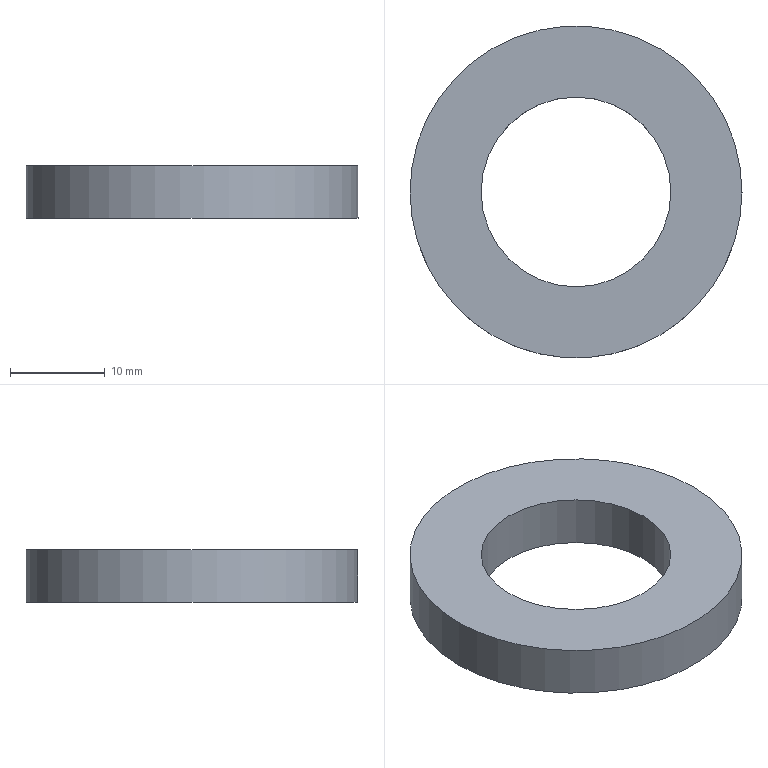Part | NX | 1 solid | 4 faces | box 35 x 35 x 5.5 mm | volume 3564 mm3 | plane 2 | cylinder 2 | commonest cylinder face diameters 20 x1 35 x1
STEP:
#1=CARTESIAN_POINT('',(17.5,0.,5.5));
#2=VERTEX_POINT('',#1);
#3=CARTESIAN_POINT('',(0.,0.,5.5));
#4=DIRECTION('',(0.,0.,1.));
#5=DIRECTION('',(1.,0.,0.));
#6=AXIS2_PLACEMENT_3D('',#3,#4,#5);
#7=CIRCLE('',#6,17.5);
#8=EDGE_CURVE('',#2,#2,#7,.T.);
#9=ORIENTED_EDGE('',*,*,#8,.T.);
#10=EDGE_LOOP('',(#9));
#11=FACE_BOUND('',#10,.T.);
#12=CARTESIAN_POINT('',(10.,0.,5.5));
#13=VERTEX_POINT('',#12);
#14=CARTESIAN_POINT('',(0.,0.,5.5));
#15=DIRECTION('',(0.,0.,1.));
#16=DIRECTION('',(1.,0.,0.));
#17=AXIS2_PLACEMENT_3D('',#14,#15,#16);
#18=CIRCLE('',#17,10.);
#19=EDGE_CURVE('',#13,#13,#18,.T.);
#20=ORIENTED_EDGE('',*,*,#19,.F.);
#21=EDGE_LOOP('',(#20));
#22=FACE_BOUND('',#21,.T.);
#23=CARTESIAN_POINT('',(0.,0.,5.5));
#24=DIRECTION('',(0.,0.,1.));
#25=DIRECTION('',(1.,0.,0.));
#26=AXIS2_PLACEMENT_3D('',#23,#24,#25);
#27=PLANE('',#26);
#28=ADVANCED_FACE('',(#11,#22),#27,.T.);
#29=CARTESIAN_POINT('',(17.5,0.,0.));
#30=VERTEX_POINT('',#29);
#31=CARTESIAN_POINT('',(0.,0.,0.));
#32=DIRECTION('',(0.,0.,1.));
#33=DIRECTION('',(1.,0.,0.));
#34=AXIS2_PLACEMENT_3D('',#31,#32,#33);
#35=CIRCLE('',#34,17.5);
#36=EDGE_CURVE('',#30,#30,#35,.T.);
#37=ORIENTED_EDGE('',*,*,#36,.F.);
#38=EDGE_LOOP('',(#37));
#39=FACE_BOUND('',#38,.T.);
#40=CARTESIAN_POINT('',(10.,0.,0.));
#41=VERTEX_POINT('',#40);
#42=CARTESIAN_POINT('',(0.,0.,0.));
#43=DIRECTION('',(0.,0.,1.));
#44=DIRECTION('',(1.,0.,0.));
#45=AXIS2_PLACEMENT_3D('',#42,#43,#44);
#46=CIRCLE('',#45,10.);
#47=EDGE_CURVE('',#41,#41,#46,.T.);
#48=ORIENTED_EDGE('',*,*,#47,.T.);
#49=EDGE_LOOP('',(#48));
#50=FACE_BOUND('',#49,.T.);
#51=CARTESIAN_POINT('',(0.,0.,0.));
#52=DIRECTION('',(0.,0.,1.));
#53=DIRECTION('',(1.,0.,0.));
#54=AXIS2_PLACEMENT_3D('',#51,#52,#53);
#55=PLANE('',#54);
#56=ADVANCED_FACE('',(#39,#50),#55,.F.);
#57=ORIENTED_EDGE('',*,*,#8,.F.);
#58=EDGE_LOOP('',(#57));
#59=FACE_BOUND('',#58,.T.);
#60=ORIENTED_EDGE('',*,*,#36,.T.);
#61=EDGE_LOOP('',(#60));
#62=FACE_BOUND('',#61,.T.);
#63=CARTESIAN_POINT('',(0.,0.,5.5));
#64=DIRECTION('',(0.,0.,-1.));
#65=DIRECTION('',(-1.,0.,0.));
#66=AXIS2_PLACEMENT_3D('',#63,#64,#65);
#67=CYLINDRICAL_SURFACE('',#66,17.5);
#68=ADVANCED_FACE('',(#59,#62),#67,.T.);
#69=ORIENTED_EDGE('',*,*,#19,.T.);
#70=EDGE_LOOP('',(#69));
#71=FACE_BOUND('',#70,.T.);
#72=ORIENTED_EDGE('',*,*,#47,.F.);
#73=EDGE_LOOP('',(#72));
#74=FACE_BOUND('',#73,.T.);
#75=CARTESIAN_POINT('',(0.,0.,5.5));
#76=DIRECTION('',(0.,0.,-1.));
#77=DIRECTION('',(-1.,0.,0.));
#78=AXIS2_PLACEMENT_3D('',#75,#76,#77);
#79=CYLINDRICAL_SURFACE('',#78,10.);
#80=ADVANCED_FACE('',(#71,#74),#79,.F.);
#81=CLOSED_SHELL('',(#28,#56,#68,#80));
#82=MANIFOLD_SOLID_BREP('',#81);
#83=(LENGTH_UNIT()NAMED_UNIT(*)SI_UNIT(.MILLI.,.METRE.));
#84=UNCERTAINTY_MEASURE_WITH_UNIT(LENGTH_MEASURE(0.00001),#83,'','');
#85=(NAMED_UNIT(*)PLANE_ANGLE_UNIT()SI_UNIT($,.RADIAN.));
#86=(NAMED_UNIT(*)SI_UNIT($,.STERADIAN.)SOLID_ANGLE_UNIT());
#87=(GEOMETRIC_REPRESENTATION_CONTEXT(3)GLOBAL_UNCERTAINTY_ASSIGNED_CONTEXT((#84))GLOBAL_UNIT_ASSIGNED_CONTEXT((#83,#85,#86))REPRESENTATION_CONTEXT('',''));
#88=ADVANCED_BREP_SHAPE_REPRESENTATION('',(#82),#87);